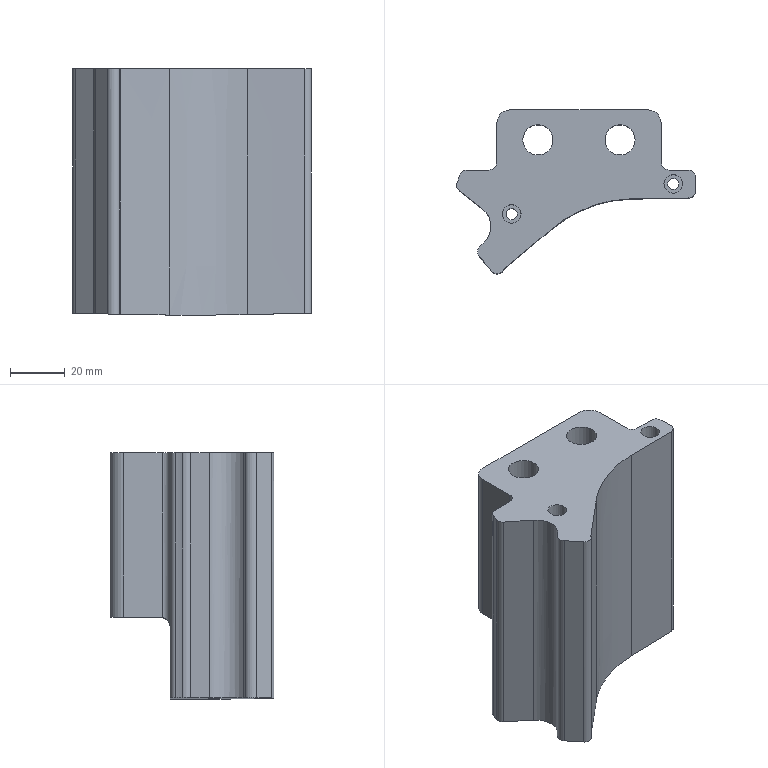Part | STEP file | gslz 2016.10.28-10_id3118_x_t | 1 solid | 42 faces | box 87.187 x 59.877 x 90 mm | volume 187380 mm3 | cylinder 22 | plane 17 | other 3 | commonest cylinder face diameters 5 x6 6 x3 4.1 x2 6.8 x2 10 x2 11 x2